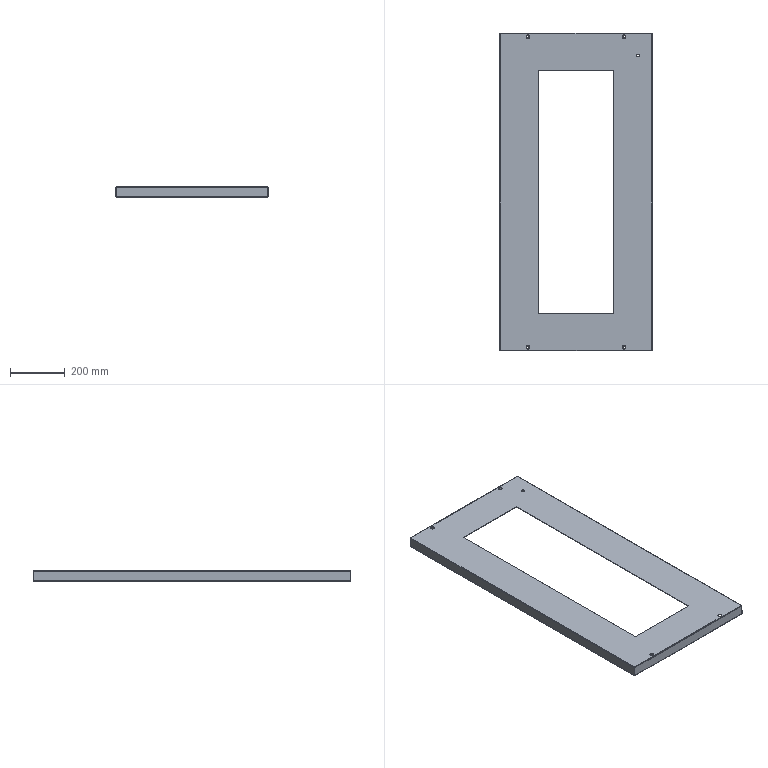Part | STEP file | SX-019-01 | 1 solid | 92 faces | box 553.501 x 1156 x 39 mm | volume 1189925 mm3 | plane 46 | cylinder 34 | spline 12 | commonest cylinder face diameters 0.4 x8 4.4 x8 8 x8 14 x8 10 x2